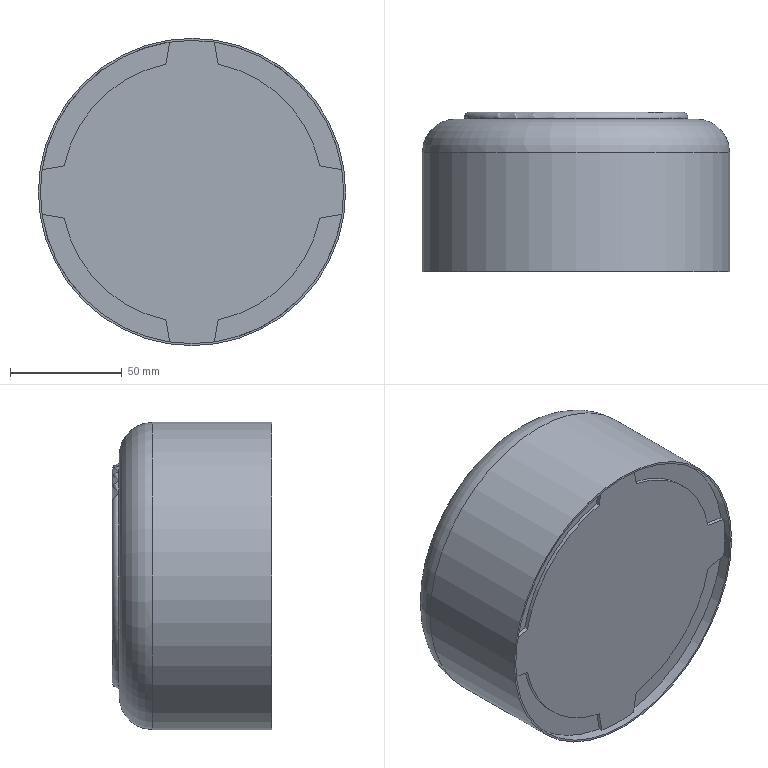Part | STEP file | 6 | 1 solid | 27 faces | box 137.76 x 71.5 x 137.76 mm | volume 961193 mm3 | plane 17 | cylinder 7 | torus 3 | commonest cylinder face diameters 117 x4 100.5 x1 136 x1 137.76 x1